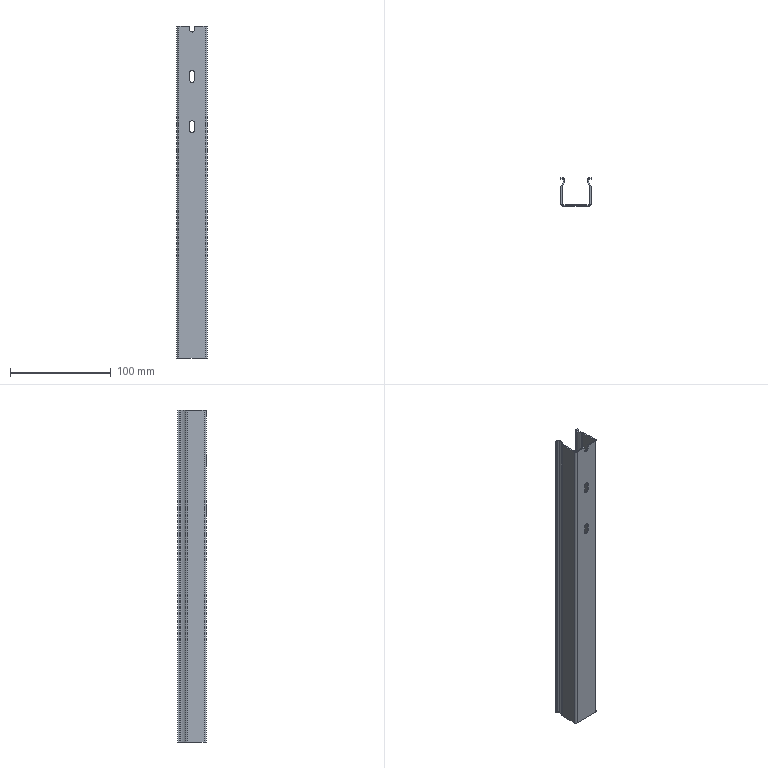Part | SolidWorks | features BaseBody 1 | 1 solid | 47 faces | box 30 x 28 x 330 mm | volume 35652 mm3 | cylinder 26 | plane 21 | commonest cylinder face diameters 5 x8 2 x3 4.5 x3 1.5 x2 3.5 x2 4 x2
STEP:
#1=CARTESIAN_POINT('',(-2.5,-12.75,-103.5));
#2=VERTEX_POINT('',#1);
#3=CARTESIAN_POINT('',(-2.5,-12.75,-96.5));
#4=VERTEX_POINT('',#3);
#5=CARTESIAN_POINT('',(-2.5,-12.75,-96.5));
#6=DIRECTION('',(0.,0.,1.));
#7=VECTOR('',#6,1000.);
#8=LINE('',#5,#7);
#9=EDGE_CURVE('',#2,#4,#8,.T.);
#10=ORIENTED_EDGE('',*,*,#9,.T.);
#11=CARTESIAN_POINT('',(-2.5,-14.,-96.5));
#12=VERTEX_POINT('',#11);
#13=CARTESIAN_POINT('',(-2.5,14.001,-96.5));
#14=DIRECTION('',(0.,-1.,0.));
#15=VECTOR('',#14,1000.);
#16=LINE('',#13,#15);
#17=EDGE_CURVE('',#4,#12,#16,.T.);
#18=ORIENTED_EDGE('',*,*,#17,.T.);
#19=CARTESIAN_POINT('',(-2.5,-14.,-103.5));
#20=VERTEX_POINT('',#19);
#21=CARTESIAN_POINT('',(-2.5,-14.,-96.5));
#22=DIRECTION('',(0.,0.,-1.));
#23=VECTOR('',#22,1000.);
#24=LINE('',#21,#23);
#25=EDGE_CURVE('',#12,#20,#24,.T.);
#26=ORIENTED_EDGE('',*,*,#25,.T.);
#27=CARTESIAN_POINT('',(-2.5,14.001,-103.5));
#28=DIRECTION('',(0.,-1.,0.));
#29=VECTOR('',#28,1000.);
#30=LINE('',#27,#29);
#31=EDGE_CURVE('',#2,#20,#30,.T.);
#32=ORIENTED_EDGE('',*,*,#31,.F.);
#33=EDGE_LOOP('',(#10,#18,#26,#32));
#34=FACE_OUTER_BOUND('',#33,.T.);
#35=CARTESIAN_POINT('',(-2.5,14.001,-96.5));
#36=DIRECTION('',(-1.,0.,0.));
#37=DIRECTION('',(0.,0.,1.));
#38=AXIS2_PLACEMENT_3D('',#35,#36,#37);
#39=PLANE('',#38);
#40=ADVANCED_FACE('',(#34),#39,.F.);
#41=CARTESIAN_POINT('',(0.,-12.75,-106.));
#42=VERTEX_POINT('',#41);
#43=CARTESIAN_POINT('',(0.,-14.,-106.));
#44=VERTEX_POINT('',#43);
#45=CARTESIAN_POINT('',(0.,14.001,-106.));
#46=DIRECTION('',(0.,-1.,0.));
#47=VECTOR('',#46,1000.);
#48=LINE('',#45,#47);
#49=EDGE_CURVE('',#42,#44,#48,.T.);
#50=ORIENTED_EDGE('',*,*,#49,.F.);
#51=CARTESIAN_POINT('',(0.,-12.75,-103.5));
#52=DIRECTION('',(0.,1.,0.));
#53=DIRECTION('',(0.,0.,-1.));
#54=AXIS2_PLACEMENT_3D('',#51,#52,#53);
#55=CIRCLE('',#54,2.5);
#56=EDGE_CURVE('',#42,#2,#55,.T.);
#57=ORIENTED_EDGE('',*,*,#56,.T.);
#58=ORIENTED_EDGE('',*,*,#31,.T.);
#59=CARTESIAN_POINT('',(0.,-14.,-103.5));
#60=DIRECTION('',(0.,-1.,0.));
#61=DIRECTION('',(0.,0.,-1.));
#62=AXIS2_PLACEMENT_3D('',#59,#60,#61);
#63=CIRCLE('',#62,2.5);
#64=EDGE_CURVE('',#20,#44,#63,.T.);
#65=ORIENTED_EDGE('',*,*,#64,.T.);
#66=EDGE_LOOP('',(#50,#57,#58,#65));
#67=FACE_OUTER_BOUND('',#66,.T.);
#68=CARTESIAN_POINT('',(0.,14.001,-103.5));
#69=DIRECTION('',(0.,-1.,0.));
#70=DIRECTION('',(0.,0.,-1.));
#71=AXIS2_PLACEMENT_3D('',#68,#69,#70);
#72=CYLINDRICAL_SURFACE('',#71,2.5);
#73=ADVANCED_FACE('',(#67),#72,.F.);
#74=CARTESIAN_POINT('',(2.5,-12.75,-96.5));
#75=VERTEX_POINT('',#74);
#76=CARTESIAN_POINT('',(2.5,-12.75,-103.5));
#77=VERTEX_POINT('',#76);
#78=CARTESIAN_POINT('',(2.5,-12.75,-96.5));
#79=DIRECTION('',(0.,0.,-1.));
#80=VECTOR('',#79,1000.);
#81=LINE('',#78,#80);
#82=EDGE_CURVE('',#75,#77,#81,.T.);
#83=ORIENTED_EDGE('',*,*,#82,.T.);
#84=CARTESIAN_POINT('',(2.5,-14.,-103.5));
#85=VERTEX_POINT('',#84);
#86=CARTESIAN_POINT('',(2.5,14.001,-103.5));
#87=DIRECTION('',(0.,-1.,0.));
#88=VECTOR('',#87,1000.);
#89=LINE('',#86,#88);
#90=EDGE_CURVE('',#77,#85,#89,.T.);
#91=ORIENTED_EDGE('',*,*,#90,.T.);
#92=CARTESIAN_POINT('',(2.5,-14.,-96.5));
#93=VERTEX_POINT('',#92);
#94=CARTESIAN_POINT('',(2.5,-14.,-96.5));
#95=DIRECTION('',(0.,0.,1.));
#96=VECTOR('',#95,1000.);
#97=LINE('',#94,#96);
#98=EDGE_CURVE('',#85,#93,#97,.T.);
#99=ORIENTED_EDGE('',*,*,#98,.T.);
#100=CARTESIAN_POINT('',(2.5,14.001,-96.5));
#101=DIRECTION('',(0.,-1.,0.));
#102=VECTOR('',#101,1000.);
#103=LINE('',#100,#102);
#104=EDGE_CURVE('',#75,#93,#103,.T.);
#105=ORIENTED_EDGE('',*,*,#104,.F.);
#106=EDGE_LOOP('',(#83,#91,#99,#105));
#107=FACE_OUTER_BOUND('',#106,.T.);
#108=CARTESIAN_POINT('',(2.5,14.001,-96.5));
#109=DIRECTION('',(1.,0.,0.));
#110=DIRECTION('',(0.,0.,1.));
#111=AXIS2_PLACEMENT_3D('',#108,#109,#110);
#112=PLANE('',#111);
#113=ADVANCED_FACE('',(#107),#112,.F.);
#114=CARTESIAN_POINT('',(0.,-12.75,-96.5));
#115=DIRECTION('',(0.,1.,0.));
#116=DIRECTION('',(0.,0.,-1.));
#117=AXIS2_PLACEMENT_3D('',#114,#115,#116);
#118=CIRCLE('',#117,2.5);
#119=EDGE_CURVE('',#4,#75,#118,.T.);
#120=ORIENTED_EDGE('',*,*,#119,.T.);
#121=ORIENTED_EDGE('',*,*,#104,.T.);
#122=CARTESIAN_POINT('',(0.,-14.,-96.5));
#123=DIRECTION('',(0.,-1.,0.));
#124=DIRECTION('',(0.,0.,-1.));
#125=AXIS2_PLACEMENT_3D('',#122,#123,#124);
#126=CIRCLE('',#125,2.5);
#127=EDGE_CURVE('',#93,#12,#126,.T.);
#128=ORIENTED_EDGE('',*,*,#127,.T.);
#129=ORIENTED_EDGE('',*,*,#17,.F.);
#130=EDGE_LOOP('',(#120,#121,#128,#129));
#131=FACE_OUTER_BOUND('',#130,.T.);
#132=CARTESIAN_POINT('',(0.,14.001,-96.5));
#133=DIRECTION('',(0.,-1.,0.));
#134=DIRECTION('',(0.,0.,-1.));
#135=AXIS2_PLACEMENT_3D('',#132,#133,#134);
#136=CYLINDRICAL_SURFACE('',#135,2.5);
#137=ADVANCED_FACE('',(#131),#136,.F.);
#138=CARTESIAN_POINT('',(-2.5,-12.75,-53.5));
#139=VERTEX_POINT('',#138);
#140=CARTESIAN_POINT('',(-2.5,-12.75,-46.5));
#141=VERTEX_POINT('',#140);
#142=CARTESIAN_POINT('',(-2.5,-12.75,-46.5));
#143=DIRECTION('',(0.,0.,1.));
#144=VECTOR('',#143,1000.);
#145=LINE('',#142,#144);
#146=EDGE_CURVE('',#139,#141,#145,.T.);
#147=ORIENTED_EDGE('',*,*,#146,.T.);
#148=CARTESIAN_POINT('',(-2.5,-14.,-46.5));
#149=VERTEX_POINT('',#148);
#150=CARTESIAN_POINT('',(-2.5,14.001,-46.5));
#151=DIRECTION('',(0.,-1.,0.));
#152=VECTOR('',#151,1000.);
#153=LINE('',#150,#152);
#154=EDGE_CURVE('',#141,#149,#153,.T.);
#155=ORIENTED_EDGE('',*,*,#154,.T.);
#156=CARTESIAN_POINT('',(-2.5,-14.,-53.5));
#157=VERTEX_POINT('',#156);
#158=CARTESIAN_POINT('',(-2.5,-14.,-46.5));
#159=DIRECTION('',(0.,0.,-1.));
#160=VECTOR('',#159,1000.);
#161=LINE('',#158,#160);
#162=EDGE_CURVE('',#149,#157,#161,.T.);
#163=ORIENTED_EDGE('',*,*,#162,.T.);
#164=CARTESIAN_POINT('',(-2.5,14.001,-53.5));
#165=DIRECTION('',(0.,-1.,0.));
#166=VECTOR('',#165,1000.);
#167=LINE('',#164,#166);
#168=EDGE_CURVE('',#139,#157,#167,.T.);
#169=ORIENTED_EDGE('',*,*,#168,.F.);
#170=EDGE_LOOP('',(#147,#155,#163,#169));
#171=FACE_OUTER_BOUND('',#170,.T.);
#172=CARTESIAN_POINT('',(-2.5,14.001,-46.5));
#173=DIRECTION('',(-1.,0.,0.));
#174=DIRECTION('',(0.,0.,1.));
#175=AXIS2_PLACEMENT_3D('',#172,#173,#174);
#176=PLANE('',#175);
#177=ADVANCED_FACE('',(#171),#176,.F.);
#178=CARTESIAN_POINT('',(0.,-12.75,-56.));
#179=VERTEX_POINT('',#178);
#180=CARTESIAN_POINT('',(0.,-14.,-56.));
#181=VERTEX_POINT('',#180);
#182=CARTESIAN_POINT('',(0.,14.001,-56.));
#183=DIRECTION('',(0.,-1.,0.));
#184=VECTOR('',#183,1000.);
#185=LINE('',#182,#184);
#186=EDGE_CURVE('',#179,#181,#185,.T.);
#187=ORIENTED_EDGE('',*,*,#186,.F.);
#188=CARTESIAN_POINT('',(0.,-12.75,-53.5));
#189=DIRECTION('',(0.,1.,0.));
#190=DIRECTION('',(0.,0.,-1.));
#191=AXIS2_PLACEMENT_3D('',#188,#189,#190);
#192=CIRCLE('',#191,2.5);
#193=EDGE_CURVE('',#179,#139,#192,.T.);
#194=ORIENTED_EDGE('',*,*,#193,.T.);
#195=ORIENTED_EDGE('',*,*,#168,.T.);
#196=CARTESIAN_POINT('',(0.,-14.,-53.5));
#197=DIRECTION('',(0.,-1.,0.));
#198=DIRECTION('',(0.,0.,-1.));
#199=AXIS2_PLACEMENT_3D('',#196,#197,#198);
#200=CIRCLE('',#199,2.5);
#201=EDGE_CURVE('',#157,#181,#200,.T.);
#202=ORIENTED_EDGE('',*,*,#201,.T.);
#203=EDGE_LOOP('',(#187,#194,#195,#202));
#204=FACE_OUTER_BOUND('',#203,.T.);
#205=CARTESIAN_POINT('',(0.,14.001,-53.5));
#206=DIRECTION('',(0.,-1.,0.));
#207=DIRECTION('',(0.,0.,-1.));
#208=AXIS2_PLACEMENT_3D('',#205,#206,#207);
#209=CYLINDRICAL_SURFACE('',#208,2.5);
#210=ADVANCED_FACE('',(#204),#209,.F.);
#211=CARTESIAN_POINT('',(2.5,-12.75,-46.5));
#212=VERTEX_POINT('',#211);
#213=CARTESIAN_POINT('',(2.5,-12.75,-53.5));
#214=VERTEX_POINT('',#213);
#215=CARTESIAN_POINT('',(2.5,-12.75,-46.5));
#216=DIRECTION('',(0.,0.,-1.));
#217=VECTOR('',#216,1000.);
#218=LINE('',#215,#217);
#219=EDGE_CURVE('',#212,#214,#218,.T.);
#220=ORIENTED_EDGE('',*,*,#219,.T.);
#221=CARTESIAN_POINT('',(2.5,-14.,-53.5));
#222=VERTEX_POINT('',#221);
#223=CARTESIAN_POINT('',(2.5,14.001,-53.5));
#224=DIRECTION('',(0.,-1.,0.));
#225=VECTOR('',#224,1000.);
#226=LINE('',#223,#225);
#227=EDGE_CURVE('',#214,#222,#226,.T.);
#228=ORIENTED_EDGE('',*,*,#227,.T.);
#229=CARTESIAN_POINT('',(2.5,-14.,-46.5));
#230=VERTEX_POINT('',#229);
#231=CARTESIAN_POINT('',(2.5,-14.,-46.5));
#232=DIRECTION('',(0.,0.,1.));
#233=VECTOR('',#232,1000.);
#234=LINE('',#231,#233);
#235=EDGE_CURVE('',#222,#230,#234,.T.);
#236=ORIENTED_EDGE('',*,*,#235,.T.);
#237=CARTESIAN_POINT('',(2.5,14.001,-46.5));
#238=DIRECTION('',(0.,-1.,0.));
#239=VECTOR('',#238,1000.);
#240=LINE('',#237,#239);
#241=EDGE_CURVE('',#212,#230,#240,.T.);
#242=ORIENTED_EDGE('',*,*,#241,.F.);
#243=EDGE_LOOP('',(#220,#228,#236,#242));
#244=FACE_OUTER_BOUND('',#243,.T.);
#245=CARTESIAN_POINT('',(2.5,14.001,-46.5));
#246=DIRECTION('',(1.,0.,0.));
#247=DIRECTION('',(0.,0.,1.));
#248=AXIS2_PLACEMENT_3D('',#245,#246,#247);
#249=PLANE('',#248);
#250=ADVANCED_FACE('',(#244),#249,.F.);
#251=CARTESIAN_POINT('',(0.,-12.75,-46.5));
#252=DIRECTION('',(0.,1.,0.));
#253=DIRECTION('',(0.,0.,-1.));
#254=AXIS2_PLACEMENT_3D('',#251,#252,#253);
#255=CIRCLE('',#254,2.5);
#256=EDGE_CURVE('',#141,#212,#255,.T.);
#257=ORIENTED_EDGE('',*,*,#256,.T.);
#258=ORIENTED_EDGE('',*,*,#241,.T.);
#259=CARTESIAN_POINT('',(0.,-14.,-46.5));
#260=DIRECTION('',(0.,-1.,0.));
#261=DIRECTION('',(0.,0.,-1.));
#262=AXIS2_PLACEMENT_3D('',#259,#260,#261);
#263=CIRCLE('',#262,2.5);
#264=EDGE_CURVE('',#230,#149,#263,.T.);
#265=ORIENTED_EDGE('',*,*,#264,.T.);
#266=ORIENTED_EDGE('',*,*,#154,.F.);
#267=EDGE_LOOP('',(#257,#258,#265,#266));
#268=FACE_OUTER_BOUND('',#267,.T.);
#269=CARTESIAN_POINT('',(0.,14.001,-46.5));
#270=DIRECTION('',(0.,-1.,0.));
#271=DIRECTION('',(0.,0.,-1.));
#272=AXIS2_PLACEMENT_3D('',#269,#270,#271);
#273=CYLINDRICAL_SURFACE('',#272,2.5);
#274=ADVANCED_FACE('',(#268),#273,.F.);
#275=CARTESIAN_POINT('',(-2.5,-14.,0.));
#276=VERTEX_POINT('',#275);
#277=CARTESIAN_POINT('',(-2.5,-14.,-3.5));
#278=VERTEX_POINT('',#277);
#279=CARTESIAN_POINT('',(-2.5,-14.,3.5));
#280=DIRECTION('',(0.,0.,-1.));
#281=VECTOR('',#280,1000.);
#282=LINE('',#279,#281);
#283=EDGE_CURVE('',#276,#278,#282,.T.);
#284=ORIENTED_EDGE('',*,*,#283,.T.);
#285=CARTESIAN_POINT('',(-2.5,-12.75,-3.5));
#286=VERTEX_POINT('',#285);
#287=CARTESIAN_POINT('',(-2.5,14.001,-3.5));
#288=DIRECTION('',(0.,-1.,0.));
#289=VECTOR('',#288,1000.);
#290=LINE('',#287,#289);
#291=EDGE_CURVE('',#286,#278,#290,.T.);
#292=ORIENTED_EDGE('',*,*,#291,.F.);
#293=CARTESIAN_POINT('',(-2.5,-12.75,0.));
#294=VERTEX_POINT('',#293);
#295=CARTESIAN_POINT('',(-2.5,-12.75,3.5));
#296=DIRECTION('',(0.,0.,1.));
#297=VECTOR('',#296,1000.);
#298=LINE('',#295,#297);
#299=EDGE_CURVE('',#286,#294,#298,.T.);
#300=ORIENTED_EDGE('',*,*,#299,.T.);
#301=CARTESIAN_POINT('',(-2.5,14.001,0.));
#302=DIRECTION('',(0.,1.,0.));
#303=VECTOR('',#302,1000.);
#304=LINE('',#301,#303);
#305=EDGE_CURVE('',#276,#294,#304,.T.);
#306=ORIENTED_EDGE('',*,*,#305,.F.);
#307=EDGE_LOOP('',(#284,#292,#300,#306));
#308=FACE_OUTER_BOUND('',#307,.T.);
#309=CARTESIAN_POINT('',(-2.5,14.001,3.5));
#310=DIRECTION('',(-1.,0.,0.));
#311=DIRECTION('',(0.,0.,1.));
#312=AXIS2_PLACEMENT_3D('',#309,#310,#311);
#313=PLANE('',#312);
#314=ADVANCED_FACE('',(#308),#313,.F.);
#315=CARTESIAN_POINT('',(2.5,-12.75,0.));
#316=VERTEX_POINT('',#315);
#317=CARTESIAN_POINT('',(2.5,-12.75,-3.5));
#318=VERTEX_POINT('',#317);
#319=CARTESIAN_POINT('',(2.5,-12.75,3.5));
#320=DIRECTION('',(0.,0.,-1.));
#321=VECTOR('',#320,1000.);
#322=LINE('',#319,#321);
#323=EDGE_CURVE('',#316,#318,#322,.T.);
#324=ORIENTED_EDGE('',*,*,#323,.T.);
#325=CARTESIAN_POINT('',(2.5,-14.,-3.5));
#326=VERTEX_POINT('',#325);
#327=CARTESIAN_POINT('',(2.5,14.001,-3.5));
#328=DIRECTION('',(0.,-1.,0.));
#329=VECTOR('',#328,1000.);
#330=LINE('',#327,#329);
#331=EDGE_CURVE('',#318,#326,#330,.T.);
#332=ORIENTED_EDGE('',*,*,#331,.T.);
#333=CARTESIAN_POINT('',(2.5,-14.,0.));
#334=VERTEX_POINT('',#333);
#335=CARTESIAN_POINT('',(2.5,-14.,3.5));
#336=DIRECTION('',(0.,0.,1.));
#337=VECTOR('',#336,1000.);
#338=LINE('',#335,#337);
#339=EDGE_CURVE('',#326,#334,#338,.T.);
#340=ORIENTED_EDGE('',*,*,#339,.T.);
#341=CARTESIAN_POINT('',(2.5,14.001,0.));
#342=DIRECTION('',(0.,-1.,0.));
#343=VECTOR('',#342,1000.);
#344=LINE('',#341,#343);
#345=EDGE_CURVE('',#316,#334,#344,.T.);
#346=ORIENTED_EDGE('',*,*,#345,.F.);
#347=EDGE_LOOP('',(#324,#332,#340,#346));
#348=FACE_OUTER_BOUND('',#347,.T.);
#349=CARTESIAN_POINT('',(2.5,14.001,3.5));
#350=DIRECTION('',(1.,0.,0.));
#351=DIRECTION('',(0.,0.,1.));
#352=AXIS2_PLACEMENT_3D('',#349,#350,#351);
#353=PLANE('',#352);
#354=ADVANCED_FACE('',(#348),#353,.F.);
#355=CARTESIAN_POINT('',(0.,-12.75,-6.));
#356=VERTEX_POINT('',#355);
#357=CARTESIAN_POINT('',(0.,-14.,-6.));
#358=VERTEX_POINT('',#357);
#359=CARTESIAN_POINT('',(0.,14.001,-6.));
#360=DIRECTION('',(0.,-1.,0.));
#361=VECTOR('',#360,1000.);
#362=LINE('',#359,#361);
#363=EDGE_CURVE('',#356,#358,#362,.T.);
#364=ORIENTED_EDGE('',*,*,#363,.F.);
#365=CARTESIAN_POINT('',(0.,-12.75,-3.5));
#366=DIRECTION('',(0.,1.,0.));
#367=DIRECTION('',(0.,0.,-1.));
#368=AXIS2_PLACEMENT_3D('',#365,#366,#367);
#369=CIRCLE('',#368,2.5);
#370=EDGE_CURVE('',#356,#286,#369,.T.);
#371=ORIENTED_EDGE('',*,*,#370,.T.);
#372=ORIENTED_EDGE('',*,*,#291,.T.);
#373=CARTESIAN_POINT('',(0.,-14.,-3.5));
#374=DIRECTION('',(0.,-1.,0.));
#375=DIRECTION('',(0.,0.,-1.));
#376=AXIS2_PLACEMENT_3D('',#373,#374,#375);
#377=CIRCLE('',#376,2.5);
#378=EDGE_CURVE('',#278,#358,#377,.T.);
#379=ORIENTED_EDGE('',*,*,#378,.T.);
#380=EDGE_LOOP('',(#364,#371,#372,#379));
#381=FACE_OUTER_BOUND('',#380,.T.);
#382=CARTESIAN_POINT('',(0.,14.001,-3.5));
#383=DIRECTION('',(0.,-1.,0.));
#384=DIRECTION('',(0.,0.,-1.));
#385=AXIS2_PLACEMENT_3D('',#382,#383,#384);
#386=CYLINDRICAL_SURFACE('',#385,2.5);
#387=ADVANCED_FACE('',(#381),#386,.F.);
#388=CARTESIAN_POINT('',(-13.,-12.75,-330.));
#389=VERTEX_POINT('',#388);
#390=CARTESIAN_POINT('',(-13.75,-12.,-330.));
#391=VERTEX_POINT('',#390);
#392=CARTESIAN_POINT('',(-13.,-12.,-330.));
#393=DIRECTION('',(0.,0.,-1.));
#394=DIRECTION('',(1.,0.,0.));
#395=AXIS2_PLACEMENT_3D('',#392,#393,#394);
#396=CIRCLE('',#395,0.75);
#397=EDGE_CURVE('',#389,#391,#396,.T.);
#398=ORIENTED_EDGE('',*,*,#397,.T.);
#399=CARTESIAN_POINT('',(-13.75,-12.,0.));
#400=VERTEX_POINT('',#399);
#401=CARTESIAN_POINT('',(-13.75,-12.,-330.));
#402=DIRECTION('',(0.,0.,1.));
#403=VECTOR('',#402,1000.);
#404=LINE('',#401,#403);
#405=EDGE_CURVE('',#391,#400,#404,.T.);
#406=ORIENTED_EDGE('',*,*,#405,.T.);
#407=CARTESIAN_POINT('',(-13.,-12.75,0.));
#408=VERTEX_POINT('',#407);
#409=CARTESIAN_POINT('',(-13.,-12.,0.));
#410=DIRECTION('',(0.,0.,1.));
#411=DIRECTION('',(1.,0.,0.));
#412=AXIS2_PLACEMENT_3D('',#409,#410,#411);
#413=CIRCLE('',#412,0.75);
#414=EDGE_CURVE('',#400,#408,#413,.T.);
#415=ORIENTED_EDGE('',*,*,#414,.T.);
#416=CARTESIAN_POINT('',(-13.,-12.75,-330.));
#417=DIRECTION('',(0.,0.,-1.));
#418=VECTOR('',#417,1000.);
#419=LINE('',#416,#418);
#420=EDGE_CURVE('',#408,#389,#419,.T.);
#421=ORIENTED_EDGE('',*,*,#420,.T.);
#422=EDGE_LOOP('',(#398,#406,#415,#421));
#423=FACE_OUTER_BOUND('',#422,.T.);
#424=CARTESIAN_POINT('',(-13.,-12.,-330.));
#425=DIRECTION('',(0.,0.,1.));
#426=DIRECTION('',(1.,0.,0.));
#427=AXIS2_PLACEMENT_3D('',#424,#425,#426);
#428=CYLINDRICAL_SURFACE('',#427,0.75);
#429=ADVANCED_FACE('',(#423),#428,.F.);
#430=CARTESIAN_POINT('',(13.75,-12.,-330.));
#431=VERTEX_POINT('',#430);
#432=CARTESIAN_POINT('',(13.,-12.75,-330.));
#433=VERTEX_POINT('',#432);
#434=CARTESIAN_POINT('',(13.,-12.,-330.));
#435=DIRECTION('',(0.,0.,-1.));
#436=DIRECTION('',(1.,0.,0.));
#437=AXIS2_PLACEMENT_3D('',#434,#435,#436);
#438=CIRCLE('',#437,0.75);
#439=EDGE_CURVE('',#431,#433,#438,.T.);
#440=ORIENTED_EDGE('',*,*,#439,.T.);
#441=CARTESIAN_POINT('',(13.,-12.75,0.));
#442=VERTEX_POINT('',#441);
#443=CARTESIAN_POINT('',(13.,-12.75,-330.));
#444=DIRECTION('',(0.,0.,1.));
#445=VECTOR('',#444,1000.);
#446=LINE('',#443,#445);
#447=EDGE_CURVE('',#433,#442,#446,.T.);
#448=ORIENTED_EDGE('',*,*,#447,.T.);
#449=CARTESIAN_POINT('',(13.75,-12.,0.));
#450=VERTEX_POINT('',#449);
#451=CARTESIAN_POINT('',(13.,-12.,0.));
#452=DIRECTION('',(0.,0.,1.));
#453=DIRECTION('',(1.,0.,0.));
#454=AXIS2_PLACEMENT_3D('',#451,#452,#453);
#455=CIRCLE('',#454,0.75);
#456=EDGE_CURVE('',#442,#450,#455,.T.);
#457=ORIENTED_EDGE('',*,*,#456,.T.);
#458=CARTESIAN_POINT('',(13.75,-12.,-330.));
#459=DIRECTION('',(0.,0.,-1.));
#460=VECTOR('',#459,1000.);
#461=LINE('',#458,#460);
#462=EDGE_CURVE('',#450,#431,#461,.T.);
#463=ORIENTED_EDGE('',*,*,#462,.T.);
#464=EDGE_LOOP('',(#440,#448,#457,#463));
#465=FACE_OUTER_BOUND('',#464,.T.);
#466=CARTESIAN_POINT('',(13.,-12.,-330.));
#467=DIRECTION('',(0.,0.,1.));
#468=DIRECTION('',(1.,0.,0.));
#469=AXIS2_PLACEMENT_3D('',#466,#467,#468);
#470=CYLINDRICAL_SURFACE('',#469,0.75);
#471=ADVANCED_FACE('',(#465),#470,.F.);
#472=CARTESIAN_POINT('',(13.439,5.746,-330.));
#473=VERTEX_POINT('',#472);
#474=CARTESIAN_POINT('',(13.75,4.75,-330.));
#475=VERTEX_POINT('',#474);
#476=CARTESIAN_POINT('',(12.,4.75,-330.));
#477=DIRECTION('',(0.,0.,-1.));
#478=DIRECTION('',(1.,0.,0.));
#479=AXIS2_PLACEMENT_3D('',#476,#477,#478);
#480=CIRCLE('',#479,1.75);
#481=EDGE_CURVE('',#473,#475,#480,.T.);
#482=ORIENTED_EDGE('',*,*,#481,.T.);
#483=CARTESIAN_POINT('',(13.75,4.75,0.));
#484=VERTEX_POINT('',#483);
#485=CARTESIAN_POINT('',(13.75,4.75,-330.));
#486=DIRECTION('',(0.,0.,1.));
#487=VECTOR('',#486,1000.);
#488=LINE('',#485,#487);
#489=EDGE_CURVE('',#475,#484,#488,.T.);
#490=ORIENTED_EDGE('',*,*,#489,.T.);
#491=CARTESIAN_POINT('',(13.439,5.746,0.));
#492=VERTEX_POINT('',#491);
#493=CARTESIAN_POINT('',(12.,4.75,0.));
#494=DIRECTION('',(0.,0.,1.));
#495=DIRECTION('',(1.,0.,0.));
#496=AXIS2_PLACEMENT_3D('',#493,#494,#495);
#497=CIRCLE('',#496,1.75);
#498=EDGE_CURVE('',#484,#492,#497,.T.);
#499=ORIENTED_EDGE('',*,*,#498,.T.);
#500=CARTESIAN_POINT('',(13.439,5.746,-330.));
#501=DIRECTION('',(0.,0.,-1.));
#502=VECTOR('',#501,1000.);
#503=LINE('',#500,#502);
#504=EDGE_CURVE('',#492,#473,#503,.T.);
#505=ORIENTED_EDGE('',*,*,#504,.T.);
#506=EDGE_LOOP('',(#482,#490,#499,#505));
#507=FACE_OUTER_BOUND('',#506,.T.);
#508=CARTESIAN_POINT('',(12.,4.75,-330.));
#509=DIRECTION('',(0.,0.,1.));
#510=DIRECTION('',(1.,0.,0.));
#511=AXIS2_PLACEMENT_3D('',#508,#509,#510);
#512=CYLINDRICAL_SURFACE('',#511,1.75);
#513=ADVANCED_FACE('',(#507),#512,.F.);
#514=CARTESIAN_POINT('',(-13.75,4.75,-330.));
#515=VERTEX_POINT('',#514);
#516=CARTESIAN_POINT('',(-13.439,5.746,-330.));
#517=VERTEX_POINT('',#516);
#518=CARTESIAN_POINT('',(-12.,4.75,-330.));
#519=DIRECTION('',(0.,0.,-1.));
#520=DIRECTION('',(1.,0.,0.));
#521=AXIS2_PLACEMENT_3D('',#518,#519,#520);
#522=CIRCLE('',#521,1.75);
#523=EDGE_CURVE('',#515,#517,#522,.T.);
#524=ORIENTED_EDGE('',*,*,#523,.T.);
#525=CARTESIAN_POINT('',(-13.439,5.746,0.));
#526=VERTEX_POINT('',#525);
#527=CARTESIAN_POINT('',(-13.439,5.746,-330.));
#528=DIRECTION('',(0.,0.,1.));
#529=VECTOR('',#528,1000.);
#530=LINE('',#527,#529);
#531=EDGE_CURVE('',#517,#526,#530,.T.);
#532=ORIENTED_EDGE('',*,*,#531,.T.);
#533=CARTESIAN_POINT('',(-13.75,4.75,0.));
#534=VERTEX_POINT('',#533);
#535=CARTESIAN_POINT('',(-12.,4.75,0.));
#536=DIRECTION('',(0.,0.,1.));
#537=DIRECTION('',(1.,0.,0.));
#538=AXIS2_PLACEMENT_3D('',#535,#536,#537);
#539=CIRCLE('',#538,1.75);
#540=EDGE_CURVE('',#526,#534,#539,.T.);
#541=ORIENTED_EDGE('',*,*,#540,.T.);
#542=CARTESIAN_POINT('',(-13.75,4.75,-330.));
#543=DIRECTION('',(0.,0.,-1.));
#544=VECTOR('',#543,1000.);
#545=LINE('',#542,#544);
#546=EDGE_CURVE('',#534,#515,#545,.T.);
#547=ORIENTED_EDGE('',*,*,#546,.T.);
#548=EDGE_LOOP('',(#524,#532,#541,#547));
#549=FACE_OUTER_BOUND('',#548,.T.);
#550=CARTESIAN_POINT('',(-12.,4.75,-330.));
#551=DIRECTION('',(0.,0.,1.));
#552=DIRECTION('',(1.,0.,0.));
#553=AXIS2_PLACEMENT_3D('',#550,#551,#552);
#554=CYLINDRICAL_SURFACE('',#553,1.75);
#555=ADVANCED_FACE('',(#549),#554,.F.);
#556=CARTESIAN_POINT('',(13.55,14.,-330.));
#557=VERTEX_POINT('',#556);
#558=CARTESIAN_POINT('',(11.311,11.526,-330.));
#559=VERTEX_POINT('',#558);
#560=CARTESIAN_POINT('',(13.55,11.75,-330.));
#561=DIRECTION('',(0.,0.,1.));
#562=DIRECTION('',(1.,0.,0.));
#563=AXIS2_PLACEMENT_3D('',#560,#561,#562);
#564=CIRCLE('',#563,2.25);
#565=EDGE_CURVE('',#557,#559,#564,.T.);
#566=ORIENTED_EDGE('',*,*,#565,.T.);
#567=CARTESIAN_POINT('',(11.311,11.526,0.));
#568=VERTEX_POINT('',#567);
#569=CARTESIAN_POINT('',(11.311,11.526,-330.));
#570=DIRECTION('',(0.,0.,1.));
#571=VECTOR('',#570,1000.);
#572=LINE('',#569,#571);
#573=EDGE_CURVE('',#559,#568,#572,.T.);
#574=ORIENTED_EDGE('',*,*,#573,.T.);
#575=CARTESIAN_POINT('',(13.55,14.,0.));
#576=VERTEX_POINT('',#575);
#577=CARTESIAN_POINT('',(13.55,11.75,0.));
#578=DIRECTION('',(0.,0.,-1.));
#579=DIRECTION('',(1.,0.,0.));
#580=AXIS2_PLACEMENT_3D('',#577,#578,#579);
#581=CIRCLE('',#580,2.25);
#582=EDGE_CURVE('',#568,#576,#581,.T.);
#583=ORIENTED_EDGE('',*,*,#582,.T.);
#584=CARTESIAN_POINT('',(13.55,14.,-330.));
#585=DIRECTION('',(0.,0.,-1.));
#586=VECTOR('',#585,1000.);
#587=LINE('',#584,#586);
#588=EDGE_CURVE('',#576,#557,#587,.T.);
#589=ORIENTED_EDGE('',*,*,#588,.T.);
#590=EDGE_LOOP('',(#566,#574,#583,#589));
#591=FACE_OUTER_BOUND('',#590,.T.);
#592=CARTESIAN_POINT('',(13.55,11.75,-330.));
#593=DIRECTION('',(0.,0.,1.));
#594=DIRECTION('',(1.,0.,0.));
#595=AXIS2_PLACEMENT_3D('',#592,#593,#594);
#596=CYLINDRICAL_SURFACE('',#595,2.25);
#597=ADVANCED_FACE('',(#591),#596,.T.);
#598=CARTESIAN_POINT('',(-11.3,11.75,-330.));
#599=VERTEX_POINT('',#598);
#600=CARTESIAN_POINT('',(-11.3,11.75,0.));
#601=VERTEX_POINT('',#600);
#602=CARTESIAN_POINT('',(-11.3,11.75,-330.));
#603=DIRECTION('',(0.,0.,1.));
#604=VECTOR('',#603,1000.);
#605=LINE('',#602,#604);
#606=EDGE_CURVE('',#599,#601,#605,.T.);
#607=ORIENTED_EDGE('',*,*,#606,.F.);
#608=CARTESIAN_POINT('',(-13.55,14.,-330.));
#609=VERTEX_POINT('',#608);
#610=CARTESIAN_POINT('',(-13.55,11.75,-330.));
#611=DIRECTION('',(0.,0.,1.));
#612=DIRECTION('',(1.,0.,0.));
#613=AXIS2_PLACEMENT_3D('',#610,#611,#612);
#614=CIRCLE('',#613,2.25);
#615=EDGE_CURVE('',#599,#609,#614,.T.);
#616=ORIENTED_EDGE('',*,*,#615,.T.);
#617=CARTESIAN_POINT('',(-13.55,14.,0.));
#618=VERTEX_POINT('',#617);
#619=CARTESIAN_POINT('',(-13.55,14.,-330.));
#620=DIRECTION('',(0.,0.,1.));
#621=VECTOR('',#620,1000.);
#622=LINE('',#619,#621);
#623=EDGE_CURVE('',#609,#618,#622,.T.);
#624=ORIENTED_EDGE('',*,*,#623,.T.);
#625=CARTESIAN_POINT('',(-13.55,11.75,0.));
#626=DIRECTION('',(0.,0.,-1.));
#627=DIRECTION('',(1.,0.,0.));
#628=AXIS2_PLACEMENT_3D('',#625,#626,#627);
#629=CIRCLE('',#628,2.25);
#630=EDGE_CURVE('',#618,#601,#629,.T.);
#631=ORIENTED_EDGE('',*,*,#630,.T.);
#632=EDGE_LOOP('',(#607,#616,#624,#631));
#633=FACE_OUTER_BOUND('',#632,.T.);
#634=CARTESIAN_POINT('',(-13.55,11.75,-330.));
#635=DIRECTION('',(0.,0.,1.));
#636=DIRECTION('',(1.,0.,0.));
#637=AXIS2_PLACEMENT_3D('',#634,#635,#636);
#638=CYLINDRICAL_SURFACE('',#637,2.25);
#639=ADVANCED_FACE('',(#633),#638,.T.);
#640=CARTESIAN_POINT('',(-11.311,11.526,-330.));
#641=VERTEX_POINT('',#640);
#642=CARTESIAN_POINT('',(-23.55,12.75,-330.));
#643=DIRECTION('',(0.,0.,1.));
#644=DIRECTION('',(1.,0.,0.));
#645=AXIS2_PLACEMENT_3D('',#642,#643,#644);
#646=CIRCLE('',#645,12.3);
#647=EDGE_CURVE('',#517,#641,#646,.T.);
#648=ORIENTED_EDGE('',*,*,#647,.T.);
#649=CARTESIAN_POINT('',(-11.311,11.526,0.));
#650=VERTEX_POINT('',#649);
#651=CARTESIAN_POINT('',(-11.311,11.526,-330.));
#652=DIRECTION('',(0.,0.,-1.));
#653=VECTOR('',#652,1000.);
#654=LINE('',#651,#653);
#655=EDGE_CURVE('',#650,#641,#654,.T.);
#656=ORIENTED_EDGE('',*,*,#655,.F.);
#657=CARTESIAN_POINT('',(-23.55,12.75,0.));
#658=DIRECTION('',(0.,0.,1.));
#659=DIRECTION('',(1.,0.,0.));
#660=AXIS2_PLACEMENT_3D('',#657,#658,#659);
#661=CIRCLE('',#660,12.3);
#662=EDGE_CURVE('',#526,#650,#661,.T.);
#663=ORIENTED_EDGE('',*,*,#662,.F.);
#664=ORIENTED_EDGE('',*,*,#531,.F.);
#665=EDGE_LOOP('',(#648,#656,#663,#664));
#666=FACE_OUTER_BOUND('',#665,.T.);
#667=CARTESIAN_POINT('',(-23.55,12.75,-330.));
#668=DIRECTION('',(0.,0.,1.));
#669=DIRECTION('',(1.,0.,0.));
#670=AXIS2_PLACEMENT_3D('',#667,#668,#669);
#671=CYLINDRICAL_SURFACE('',#670,12.3);
#672=ADVANCED_FACE('',(#666),#671,.T.);
#673=CARTESIAN_POINT('',(23.55,12.75,0.));
#674=DIRECTION('',(0.,0.,1.));
#675=DIRECTION('',(1.,0.,0.));
#676=AXIS2_PLACEMENT_3D('',#673,#674,#675);
#677=CIRCLE('',#676,12.3);
#678=EDGE_CURVE('',#568,#492,#677,.T.);
#679=ORIENTED_EDGE('',*,*,#678,.F.);
#680=ORIENTED_EDGE('',*,*,#573,.F.);
#681=CARTESIAN_POINT('',(23.55,12.75,-330.));
#682=DIRECTION('',(0.,0.,1.));
#683=DIRECTION('',(1.,0.,0.));
#684=AXIS2_PLACEMENT_3D('',#681,#682,#683);
#685=CIRCLE('',#684,12.3);
#686=EDGE_CURVE('',#559,#473,#685,.T.);
#687=ORIENTED_EDGE('',*,*,#686,.T.);
#688=ORIENTED_EDGE('',*,*,#504,.F.);
#689=EDGE_LOOP('',(#679,#680,#687,#688));
#690=FACE_OUTER_BOUND('',#689,.T.);
#691=CARTESIAN_POINT('',(23.55,12.75,-330.));
#692=DIRECTION('',(0.,0.,1.));
#693=DIRECTION('',(1.,0.,0.));
#694=AXIS2_PLACEMENT_3D('',#691,#692,#693);
#695=CYLINDRICAL_SURFACE('',#694,12.3);
#696=ADVANCED_FACE('',(#690),#695,.T.);
#697=ORIENTED_EDGE('',*,*,#219,.F.);
#698=ORIENTED_EDGE('',*,*,#256,.F.);
#699=ORIENTED_EDGE('',*,*,#146,.F.);
#700=ORIENTED_EDGE('',*,*,#193,.F.);
#701=CARTESIAN_POINT('',(0.,-12.75,-53.5));
#702=DIRECTION('',(0.,1.,0.));
#703=DIRECTION('',(0.,0.,-1.));
#704=AXIS2_PLACEMENT_3D('',#701,#702,#703);
#705=CIRCLE('',#704,2.5);
#706=EDGE_CURVE('',#214,#179,#705,.T.);
#707=ORIENTED_EDGE('',*,*,#706,.F.);
#708=EDGE_LOOP('',(#697,#698,#699,#700,#707));
#709=FACE_BOUND('',#708,.T.);
#710=ORIENTED_EDGE('',*,*,#82,.F.);
#711=ORIENTED_EDGE('',*,*,#119,.F.);
#712=ORIENTED_EDGE('',*,*,#9,.F.);
#713=ORIENTED_EDGE('',*,*,#56,.F.);
#714=CARTESIAN_POINT('',(0.,-12.75,-103.5));
#715=DIRECTION('',(0.,1.,0.));
#716=DIRECTION('',(0.,0.,-1.));
#717=AXIS2_PLACEMENT_3D('',#714,#715,#716);
#718=CIRCLE('',#717,2.5);
#719=EDGE_CURVE('',#77,#42,#718,.T.);
#720=ORIENTED_EDGE('',*,*,#719,.F.);
#721=EDGE_LOOP('',(#710,#711,#712,#713,#720));
#722=FACE_BOUND('',#721,.T.);
#723=CARTESIAN_POINT('',(0.,-12.75,-3.5));
#724=DIRECTION('',(0.,1.,0.));
#725=DIRECTION('',(0.,0.,-1.));
#726=AXIS2_PLACEMENT_3D('',#723,#724,#725);
#727=CIRCLE('',#726,2.5);
#728=EDGE_CURVE('',#318,#356,#727,.T.);
#729=ORIENTED_EDGE('',*,*,#728,.F.);
#730=ORIENTED_EDGE('',*,*,#323,.F.);
#731=CARTESIAN_POINT('',(0.,-12.75,0.));
#732=DIRECTION('',(1.,0.,0.));
#733=VECTOR('',#732,1000.);
#734=LINE('',#731,#733);
#735=EDGE_CURVE('',#316,#442,#734,.T.);
#736=ORIENTED_EDGE('',*,*,#735,.T.);
#737=ORIENTED_EDGE('',*,*,#447,.F.);
#738=CARTESIAN_POINT('',(0.,-12.75,-330.));
#739=DIRECTION('',(1.,0.,0.));
#740=VECTOR('',#739,1000.);
#741=LINE('',#738,#740);
#742=EDGE_CURVE('',#389,#433,#741,.T.);
#743=ORIENTED_EDGE('',*,*,#742,.F.);
#744=ORIENTED_EDGE('',*,*,#420,.F.);
#745=CARTESIAN_POINT('',(0.,-12.75,0.));
#746=DIRECTION('',(1.,0.,0.));
#747=VECTOR('',#746,1000.);
#748=LINE('',#745,#747);
#749=EDGE_CURVE('',#408,#294,#748,.T.);
#750=ORIENTED_EDGE('',*,*,#749,.T.);
#751=ORIENTED_EDGE('',*,*,#299,.F.);
#752=ORIENTED_EDGE('',*,*,#370,.F.);
#753=EDGE_LOOP('',(#729,#730,#736,#737,#743,#744,#750,#751,#752));
#754=FACE_OUTER_BOUND('',#753,.T.);
#755=CARTESIAN_POINT('',(-15.,-12.75,-330.));
#756=DIRECTION('',(0.,-1.,0.));
#757=DIRECTION('',(0.,0.,-1.));
#758=AXIS2_PLACEMENT_3D('',#755,#756,#757);
#759=PLANE('',#758);
#760=ADVANCED_FACE('',(#709,#722,#754),#759,.F.);
#761=CARTESIAN_POINT('',(13.75,0.,0.));
#762=DIRECTION('',(0.,1.,0.));
#763=VECTOR('',#762,1000.);
#764=LINE('',#761,#763);
#765=EDGE_CURVE('',#450,#484,#764,.T.);
#766=ORIENTED_EDGE('',*,*,#765,.T.);
#767=ORIENTED_EDGE('',*,*,#489,.F.);
#768=CARTESIAN_POINT('',(13.75,0.,-330.));
#769=DIRECTION('',(0.,1.,0.));
#770=VECTOR('',#769,1000.);
#771=LINE('',#768,#770);
#772=EDGE_CURVE('',#431,#475,#771,.T.);
#773=ORIENTED_EDGE('',*,*,#772,.F.);
#774=ORIENTED_EDGE('',*,*,#462,.F.);
#775=EDGE_LOOP('',(#766,#767,#773,#774));
#776=FACE_OUTER_BOUND('',#775,.T.);
#777=CARTESIAN_POINT('',(13.75,14.,-330.));
#778=DIRECTION('',(1.,0.,0.));
#779=DIRECTION('',(0.,1.,0.));
#780=AXIS2_PLACEMENT_3D('',#777,#778,#779);
#781=PLANE('',#780);
#782=ADVANCED_FACE('',(#776),#781,.F.);
#783=CARTESIAN_POINT('',(-13.75,0.,-330.));
#784=DIRECTION('',(0.,-1.,0.));
#785=VECTOR('',#784,1000.);
#786=LINE('',#783,#785);
#787=EDGE_CURVE('',#515,#391,#786,.T.);
#788=ORIENTED_EDGE('',*,*,#787,.F.);
#789=ORIENTED_EDGE('',*,*,#546,.F.);
#790=CARTESIAN_POINT('',(-13.75,0.,0.));
#791=DIRECTION('',(0.,-1.,0.));
#792=VECTOR('',#791,1000.);
#793=LINE('',#790,#792);
#794=EDGE_CURVE('',#534,#400,#793,.T.);
#795=ORIENTED_EDGE('',*,*,#794,.T.);
#796=ORIENTED_EDGE('',*,*,#405,.F.);
#797=EDGE_LOOP('',(#788,#789,#795,#796));
#798=FACE_OUTER_BOUND('',#797,.T.);
#799=CARTESIAN_POINT('',(-13.75,14.,-330.));
#800=DIRECTION('',(-1.,0.,0.));
#801=DIRECTION('',(0.,1.,0.));
#802=AXIS2_PLACEMENT_3D('',#799,#800,#801);
#803=PLANE('',#802);
#804=ADVANCED_FACE('',(#798),#803,.F.);
#805=CARTESIAN_POINT('',(-13.,-14.,-330.));
#806=VERTEX_POINT('',#805);
#807=CARTESIAN_POINT('',(-15.,-12.,-330.));
#808=VERTEX_POINT('',#807);
#809=CARTESIAN_POINT('',(-13.,-12.,-330.));
#810=DIRECTION('',(0.,0.,-1.));
#811=DIRECTION('',(1.,0.,0.));
#812=AXIS2_PLACEMENT_3D('',#809,#810,#811);
#813=CIRCLE('',#812,2.);
#814=EDGE_CURVE('',#806,#808,#813,.T.);
#815=ORIENTED_EDGE('',*,*,#814,.F.);
#816=CARTESIAN_POINT('',(-13.,-14.,0.));
#817=VERTEX_POINT('',#816);
#818=CARTESIAN_POINT('',(-13.,-14.,-330.));
#819=DIRECTION('',(0.,0.,-1.));
#820=VECTOR('',#819,1000.);
#821=LINE('',#818,#820);
#822=EDGE_CURVE('',#817,#806,#821,.T.);
#823=ORIENTED_EDGE('',*,*,#822,.F.);
#824=CARTESIAN_POINT('',(-15.,-12.,0.));
#825=VERTEX_POINT('',#824);
#826=CARTESIAN_POINT('',(-13.,-12.,0.));
#827=DIRECTION('',(0.,0.,1.));
#828=DIRECTION('',(1.,0.,0.));
#829=AXIS2_PLACEMENT_3D('',#826,#827,#828);
#830=CIRCLE('',#829,2.);
#831=EDGE_CURVE('',#825,#817,#830,.T.);
#832=ORIENTED_EDGE('',*,*,#831,.F.);
#833=CARTESIAN_POINT('',(-15.,-12.,-330.));
#834=DIRECTION('',(0.,0.,1.));
#835=VECTOR('',#834,1000.);
#836=LINE('',#833,#835);
#837=EDGE_CURVE('',#808,#825,#836,.T.);
#838=ORIENTED_EDGE('',*,*,#837,.F.);
#839=EDGE_LOOP('',(#815,#823,#832,#838));
#840=FACE_OUTER_BOUND('',#839,.T.);
#841=CARTESIAN_POINT('',(-13.,-12.,-330.));
#842=DIRECTION('',(0.,0.,1.));
#843=DIRECTION('',(1.,0.,0.));
#844=AXIS2_PLACEMENT_3D('',#841,#842,#843);
#845=CYLINDRICAL_SURFACE('',#844,2.);
#846=ADVANCED_FACE('',(#840),#845,.T.);
#847=CARTESIAN_POINT('',(15.,-12.,-330.));
#848=VERTEX_POINT('',#847);
#849=CARTESIAN_POINT('',(13.,-14.,-330.));
#850=VERTEX_POINT('',#849);
#851=CARTESIAN_POINT('',(13.,-12.,-330.));
#852=DIRECTION('',(0.,0.,-1.));
#853=DIRECTION('',(1.,0.,0.));
#854=AXIS2_PLACEMENT_3D('',#851,#852,#853);
#855=CIRCLE('',#854,2.);
#856=EDGE_CURVE('',#848,#850,#855,.T.);
#857=ORIENTED_EDGE('',*,*,#856,.F.);
#858=CARTESIAN_POINT('',(15.,-12.,0.));
#859=VERTEX_POINT('',#858);
#860=CARTESIAN_POINT('',(15.,-12.,-330.));
#861=DIRECTION('',(0.,0.,-1.));
#862=VECTOR('',#861,1000.);
#863=LINE('',#860,#862);
#864=EDGE_CURVE('',#859,#848,#863,.T.);
#865=ORIENTED_EDGE('',*,*,#864,.F.);
#866=CARTESIAN_POINT('',(13.,-14.,0.));
#867=VERTEX_POINT('',#866);
#868=CARTESIAN_POINT('',(13.,-12.,0.));
#869=DIRECTION('',(0.,0.,1.));
#870=DIRECTION('',(1.,0.,0.));
#871=AXIS2_PLACEMENT_3D('',#868,#869,#870);
#872=CIRCLE('',#871,2.);
#873=EDGE_CURVE('',#867,#859,#872,.T.);
#874=ORIENTED_EDGE('',*,*,#873,.F.);
#875=CARTESIAN_POINT('',(13.,-14.,-330.));
#876=DIRECTION('',(0.,0.,1.));
#877=VECTOR('',#876,1000.);
#878=LINE('',#875,#877);
#879=EDGE_CURVE('',#850,#867,#878,.T.);
#880=ORIENTED_EDGE('',*,*,#879,.F.);
#881=EDGE_LOOP('',(#857,#865,#874,#880));
#882=FACE_OUTER_BOUND('',#881,.T.);
#883=CARTESIAN_POINT('',(13.,-12.,-330.));
#884=DIRECTION('',(0.,0.,1.));
#885=DIRECTION('',(1.,0.,0.));
#886=AXIS2_PLACEMENT_3D('',#883,#884,#885);
#887=CYLINDRICAL_SURFACE('',#886,2.);
#888=ADVANCED_FACE('',(#882),#887,.T.);
#889=CARTESIAN_POINT('',(14.466,6.458,-330.));
#890=VERTEX_POINT('',#889);
#891=CARTESIAN_POINT('',(15.,4.75,-330.));
#892=VERTEX_POINT('',#891);
#893=CARTESIAN_POINT('',(12.,4.75,-330.));
#894=DIRECTION('',(0.,0.,-1.));
#895=DIRECTION('',(1.,0.,0.));
#896=AXIS2_PLACEMENT_3D('',#893,#894,#895);
#897=CIRCLE('',#896,3.);
#898=EDGE_CURVE('',#890,#892,#897,.T.);
#899=ORIENTED_EDGE('',*,*,#898,.F.);
#900=CARTESIAN_POINT('',(14.466,6.458,0.));
#901=VERTEX_POINT('',#900);
#902=CARTESIAN_POINT('',(14.466,6.458,-330.));
#903=DIRECTION('',(0.,0.,-1.));
#904=VECTOR('',#903,1000.);
#905=LINE('',#902,#904);
#906=EDGE_CURVE('',#901,#890,#905,.T.);
#907=ORIENTED_EDGE('',*,*,#906,.F.);
#908=CARTESIAN_POINT('',(15.,4.75,0.));
#909=VERTEX_POINT('',#908);
#910=CARTESIAN_POINT('',(12.,4.75,0.));
#911=DIRECTION('',(0.,0.,1.));
#912=DIRECTION('',(1.,0.,0.));
#913=AXIS2_PLACEMENT_3D('',#910,#911,#912);
#914=CIRCLE('',#913,3.);
#915=EDGE_CURVE('',#909,#901,#914,.T.);
#916=ORIENTED_EDGE('',*,*,#915,.F.);
#917=CARTESIAN_POINT('',(15.,4.75,0.));
#918=DIRECTION('',(0.,0.,1.));
#919=VECTOR('',#918,1000.);
#920=LINE('',#917,#919);
#921=EDGE_CURVE('',#892,#909,#920,.T.);
#922=ORIENTED_EDGE('',*,*,#921,.F.);
#923=EDGE_LOOP('',(#899,#907,#916,#922));
#924=FACE_OUTER_BOUND('',#923,.T.);
#925=CARTESIAN_POINT('',(12.,4.75,-330.));
#926=DIRECTION('',(0.,0.,1.));
#927=DIRECTION('',(1.,0.,0.));
#928=AXIS2_PLACEMENT_3D('',#925,#926,#927);
#929=CYLINDRICAL_SURFACE('',#928,3.);
#930=ADVANCED_FACE('',(#924),#929,.T.);
#931=CARTESIAN_POINT('',(-15.,4.75,-330.));
#932=VERTEX_POINT('',#931);
#933=CARTESIAN_POINT('',(-14.466,6.458,-330.));
#934=VERTEX_POINT('',#933);
#935=CARTESIAN_POINT('',(-12.,4.75,-330.));
#936=DIRECTION('',(0.,0.,-1.));
#937=DIRECTION('',(1.,0.,0.));
#938=AXIS2_PLACEMENT_3D('',#935,#936,#937);
#939=CIRCLE('',#938,3.);
#940=EDGE_CURVE('',#932,#934,#939,.T.);
#941=ORIENTED_EDGE('',*,*,#940,.F.);
#942=CARTESIAN_POINT('',(-15.,4.75,0.));
#943=VERTEX_POINT('',#942);
#944=CARTESIAN_POINT('',(-15.,4.75,-330.));
#945=DIRECTION('',(0.,0.,-1.));
#946=VECTOR('',#945,1000.);
#947=LINE('',#944,#946);
#948=EDGE_CURVE('',#943,#932,#947,.T.);
#949=ORIENTED_EDGE('',*,*,#948,.F.);
#950=CARTESIAN_POINT('',(-14.466,6.458,0.));
#951=VERTEX_POINT('',#950);
#952=CARTESIAN_POINT('',(-12.,4.75,0.));
#953=DIRECTION('',(0.,0.,1.));
#954=DIRECTION('',(1.,0.,0.));
#955=AXIS2_PLACEMENT_3D('',#952,#953,#954);
#956=CIRCLE('',#955,3.);
#957=EDGE_CURVE('',#951,#943,#956,.T.);
#958=ORIENTED_EDGE('',*,*,#957,.F.);
#959=CARTESIAN_POINT('',(-14.466,6.458,-330.));
#960=DIRECTION('',(0.,0.,1.));
#961=VECTOR('',#960,1000.);
#962=LINE('',#959,#961);
#963=EDGE_CURVE('',#934,#951,#962,.T.);
#964=ORIENTED_EDGE('',*,*,#963,.F.);
#965=EDGE_LOOP('',(#941,#949,#958,#964));
#966=FACE_OUTER_BOUND('',#965,.T.);
#967=CARTESIAN_POINT('',(-12.,4.75,-330.));
#968=DIRECTION('',(0.,0.,1.));
#969=DIRECTION('',(1.,0.,0.));
#970=AXIS2_PLACEMENT_3D('',#967,#968,#969);
#971=CYLINDRICAL_SURFACE('',#970,3.);
#972=ADVANCED_FACE('',(#966),#971,.T.);
#973=CARTESIAN_POINT('',(13.55,12.75,-330.));
#974=VERTEX_POINT('',#973);
#975=CARTESIAN_POINT('',(12.555,11.65,-330.));
#976=VERTEX_POINT('',#975);
#977=CARTESIAN_POINT('',(13.55,11.75,-330.));
#978=DIRECTION('',(0.,0.,1.));
#979=DIRECTION('',(1.,0.,0.));
#980=AXIS2_PLACEMENT_3D('',#977,#978,#979);
#981=CIRCLE('',#980,1.);
#982=EDGE_CURVE('',#974,#976,#981,.T.);
#983=ORIENTED_EDGE('',*,*,#982,.F.);
#984=CARTESIAN_POINT('',(13.55,12.75,0.));
#985=VERTEX_POINT('',#984);
#986=CARTESIAN_POINT('',(13.55,12.75,-330.));
#987=DIRECTION('',(0.,0.,-1.));
#988=VECTOR('',#987,1000.);
#989=LINE('',#986,#988);
#990=EDGE_CURVE('',#985,#974,#989,.T.);
#991=ORIENTED_EDGE('',*,*,#990,.F.);
#992=CARTESIAN_POINT('',(12.555,11.65,0.));
#993=VERTEX_POINT('',#992);
#994=CARTESIAN_POINT('',(13.55,11.75,0.));
#995=DIRECTION('',(0.,0.,-1.));
#996=DIRECTION('',(1.,0.,0.));
#997=AXIS2_PLACEMENT_3D('',#994,#995,#996);
#998=CIRCLE('',#997,1.);
#999=EDGE_CURVE('',#993,#985,#998,.T.);
#1000=ORIENTED_EDGE('',*,*,#999,.F.);
#1001=CARTESIAN_POINT('',(12.555,11.65,-330.));
#1002=DIRECTION('',(0.,0.,1.));
#1003=VECTOR('',#1002,1000.);
#1004=LINE('',#1001,#1003);
#1005=EDGE_CURVE('',#976,#993,#1004,.T.);
#1006=ORIENTED_EDGE('',*,*,#1005,.F.);
#1007=EDGE_LOOP('',(#983,#991,#1000,#1006));
#1008=FACE_OUTER_BOUND('',#1007,.T.);
#1009=CARTESIAN_POINT('',(13.55,11.75,-330.));
#1010=DIRECTION('',(0.,0.,1.));
#1011=DIRECTION('',(1.,0.,0.));
#1012=AXIS2_PLACEMENT_3D('',#1009,#1010,#1011);
#1013=CYLINDRICAL_SURFACE('',#1012,1.);
#1014=ADVANCED_FACE('',(#1008),#1013,.F.);
#1015=CARTESIAN_POINT('',(-12.55,11.75,-330.));
#1016=VERTEX_POINT('',#1015);
#1017=CARTESIAN_POINT('',(-12.55,11.75,0.));
#1018=VERTEX_POINT('',#1017);
#1019=CARTESIAN_POINT('',(-12.55,11.75,-330.));
#1020=DIRECTION('',(0.,0.,1.));
#1021=VECTOR('',#1020,1000.);
#1022=LINE('',#1019,#1021);
#1023=EDGE_CURVE('',#1016,#1018,#1022,.T.);
#1024=ORIENTED_EDGE('',*,*,#1023,.F.);
#1025=CARTESIAN_POINT('',(-12.555,11.65,-330.));
#1026=VERTEX_POINT('',#1025);
#1027=CARTESIAN_POINT('',(-13.55,11.75,-330.));
#1028=DIRECTION('',(0.,0.,1.));
#1029=DIRECTION('',(1.,0.,0.));
#1030=AXIS2_PLACEMENT_3D('',#1027,#1028,#1029);
#1031=CIRCLE('',#1030,1.);
#1032=EDGE_CURVE('',#1026,#1016,#1031,.T.);
#1033=ORIENTED_EDGE('',*,*,#1032,.F.);
#1034=CARTESIAN_POINT('',(-12.555,11.65,0.));
#1035=VERTEX_POINT('',#1034);
#1036=CARTESIAN_POINT('',(-12.555,11.65,-330.));
#1037=DIRECTION('',(0.,0.,-1.));
#1038=VECTOR('',#1037,1000.);
#1039=LINE('',#1036,#1038);
#1040=EDGE_CURVE('',#1035,#1026,#1039,.T.);
#1041=ORIENTED_EDGE('',*,*,#1040,.F.);
#1042=CARTESIAN_POINT('',(-13.55,11.75,0.));
#1043=DIRECTION('',(0.,0.,-1.));
#1044=DIRECTION('',(1.,0.,0.));
#1045=AXIS2_PLACEMENT_3D('',#1042,#1043,#1044);
#1046=CIRCLE('',#1045,1.);
#1047=EDGE_CURVE('',#1018,#1035,#1046,.T.);
#1048=ORIENTED_EDGE('',*,*,#1047,.F.);
#1049=EDGE_LOOP('',(#1024,#1033,#1041,#1048));
#1050=FACE_OUTER_BOUND('',#1049,.T.);
#1051=CARTESIAN_POINT('',(-13.55,11.75,-330.));
#1052=DIRECTION('',(0.,0.,1.));
#1053=DIRECTION('',(1.,0.,0.));
#1054=AXIS2_PLACEMENT_3D('',#1051,#1052,#1053);
#1055=CYLINDRICAL_SURFACE('',#1054,1.);
#1056=ADVANCED_FACE('',(#1050),#1055,.F.);
#1057=CARTESIAN_POINT('',(-13.55,12.75,-330.));
#1058=VERTEX_POINT('',#1057);
#1059=CARTESIAN_POINT('',(-15.,12.75,-330.));
#1060=VERTEX_POINT('',#1059);
#1061=CARTESIAN_POINT('',(-15.,12.75,-330.));
#1062=DIRECTION('',(-1.,0.,0.));
#1063=VECTOR('',#1062,1000.);
#1064=LINE('',#1061,#1063);
#1065=EDGE_CURVE('',#1058,#1060,#1064,.T.);
#1066=ORIENTED_EDGE('',*,*,#1065,.F.);
#1067=CARTESIAN_POINT('',(-13.55,12.75,0.));
#1068=VERTEX_POINT('',#1067);
#1069=CARTESIAN_POINT('',(-13.55,12.75,0.));
#1070=DIRECTION('',(0.,0.,1.));
#1071=VECTOR('',#1070,1000.);
#1072=LINE('',#1069,#1071);
#1073=EDGE_CURVE('',#1058,#1068,#1072,.T.);
#1074=ORIENTED_EDGE('',*,*,#1073,.T.);
#1075=CARTESIAN_POINT('',(-15.,12.75,0.));
#1076=VERTEX_POINT('',#1075);
#1077=CARTESIAN_POINT('',(-15.,12.75,0.));
#1078=DIRECTION('',(-1.,0.,0.));
#1079=VECTOR('',#1078,1000.);
#1080=LINE('',#1077,#1079);
#1081=EDGE_CURVE('',#1068,#1076,#1080,.T.);
#1082=ORIENTED_EDGE('',*,*,#1081,.T.);
#1083=CARTESIAN_POINT('',(-15.,12.75,-330.));
#1084=DIRECTION('',(0.,0.,1.));
#1085=VECTOR('',#1084,1000.);
#1086=LINE('',#1083,#1085);
#1087=EDGE_CURVE('',#1060,#1076,#1086,.T.);
#1088=ORIENTED_EDGE('',*,*,#1087,.F.);
#1089=EDGE_LOOP('',(#1066,#1074,#1082,#1088));
#1090=FACE_OUTER_BOUND('',#1089,.T.);
#1091=CARTESIAN_POINT('',(-15.,12.75,-330.));
#1092=DIRECTION('',(0.,1.,0.));
#1093=DIRECTION('',(1.,0.,0.));
#1094=AXIS2_PLACEMENT_3D('',#1091,#1092,#1093);
#1095=PLANE('',#1094);
#1096=ADVANCED_FACE('',(#1090),#1095,.F.);
#1097=CARTESIAN_POINT('',(-23.55,12.75,-330.));
#1098=DIRECTION('',(0.,0.,1.));
#1099=DIRECTION('',(-1.,0.,0.));
#1100=AXIS2_PLACEMENT_3D('',#1097,#1098,#1099);
#1101=CIRCLE('',#1100,11.05);
#1102=EDGE_CURVE('',#934,#1026,#1101,.T.);
#1103=ORIENTED_EDGE('',*,*,#1102,.F.);
#1104=ORIENTED_EDGE('',*,*,#963,.T.);
#1105=CARTESIAN_POINT('',(-23.55,12.75,0.));
#1106=DIRECTION('',(0.,0.,1.));
#1107=DIRECTION('',(-1.,0.,0.));
#1108=AXIS2_PLACEMENT_3D('',#1105,#1106,#1107);
#1109=CIRCLE('',#1108,11.05);
#1110=EDGE_CURVE('',#951,#1035,#1109,.T.);
#1111=ORIENTED_EDGE('',*,*,#1110,.T.);
#1112=ORIENTED_EDGE('',*,*,#1040,.T.);
#1113=EDGE_LOOP('',(#1103,#1104,#1111,#1112));
#1114=FACE_OUTER_BOUND('',#1113,.T.);
#1115=CARTESIAN_POINT('',(-23.55,12.75,-330.));
#1116=DIRECTION('',(0.,0.,1.));
#1117=DIRECTION('',(1.,0.,0.));
#1118=AXIS2_PLACEMENT_3D('',#1115,#1116,#1117);
#1119=CYLINDRICAL_SURFACE('',#1118,11.05);
#1120=ADVANCED_FACE('',(#1114),#1119,.F.);
#1121=CARTESIAN_POINT('',(15.,12.75,0.));
#1122=VERTEX_POINT('',#1121);
#1123=CARTESIAN_POINT('',(15.,12.75,0.));
#1124=DIRECTION('',(-1.,0.,0.));
#1125=VECTOR('',#1124,1000.);
#1126=LINE('',#1123,#1125);
#1127=EDGE_CURVE('',#1122,#985,#1126,.T.);
#1128=ORIENTED_EDGE('',*,*,#1127,.T.);
#1129=ORIENTED_EDGE('',*,*,#990,.T.);
#1130=CARTESIAN_POINT('',(15.,12.75,-330.));
#1131=VERTEX_POINT('',#1130);
#1132=CARTESIAN_POINT('',(15.,12.75,-330.));
#1133=DIRECTION('',(-1.,0.,0.));
#1134=VECTOR('',#1133,1000.);
#1135=LINE('',#1132,#1134);
#1136=EDGE_CURVE('',#1131,#974,#1135,.T.);
#1137=ORIENTED_EDGE('',*,*,#1136,.F.);
#1138=CARTESIAN_POINT('',(15.,12.75,-330.));
#1139=DIRECTION('',(0.,0.,1.));
#1140=VECTOR('',#1139,1000.);
#1141=LINE('',#1138,#1140);
#1142=EDGE_CURVE('',#1131,#1122,#1141,.T.);
#1143=ORIENTED_EDGE('',*,*,#1142,.T.);
#1144=EDGE_LOOP('',(#1128,#1129,#1137,#1143));
#1145=FACE_OUTER_BOUND('',#1144,.T.);
#1146=CARTESIAN_POINT('',(15.,12.75,-330.));
#1147=DIRECTION('',(0.,1.,0.));
#1148=DIRECTION('',(1.,0.,0.));
#1149=AXIS2_PLACEMENT_3D('',#1146,#1147,#1148);
#1150=PLANE('',#1149);
#1151=ADVANCED_FACE('',(#1145),#1150,.F.);
#1152=CARTESIAN_POINT('',(23.55,12.75,0.));
#1153=DIRECTION('',(0.,0.,1.));
#1154=DIRECTION('',(1.,0.,0.));
#1155=AXIS2_PLACEMENT_3D('',#1152,#1153,#1154);
#1156=CIRCLE('',#1155,11.05);
#1157=EDGE_CURVE('',#993,#901,#1156,.T.);
#1158=ORIENTED_EDGE('',*,*,#1157,.T.);
#1159=ORIENTED_EDGE('',*,*,#906,.T.);
#1160=CARTESIAN_POINT('',(23.55,12.75,-330.));
#1161=DIRECTION('',(0.,0.,1.));
#1162=DIRECTION('',(1.,0.,0.));
#1163=AXIS2_PLACEMENT_3D('',#1160,#1161,#1162);
#1164=CIRCLE('',#1163,11.05);
#1165=EDGE_CURVE('',#976,#890,#1164,.T.);
#1166=ORIENTED_EDGE('',*,*,#1165,.F.);
#1167=ORIENTED_EDGE('',*,*,#1005,.T.);
#1168=EDGE_LOOP('',(#1158,#1159,#1166,#1167));
#1169=FACE_OUTER_BOUND('',#1168,.T.);
#1170=CARTESIAN_POINT('',(23.55,12.75,-330.));
#1171=DIRECTION('',(0.,0.,1.));
#1172=DIRECTION('',(1.,0.,0.));
#1173=AXIS2_PLACEMENT_3D('',#1170,#1171,#1172);
#1174=CYLINDRICAL_SURFACE('',#1173,11.05);
#1175=ADVANCED_FACE('',(#1169),#1174,.F.);
#1176=ORIENTED_EDGE('',*,*,#305,.T.);
#1177=ORIENTED_EDGE('',*,*,#749,.F.);
#1178=ORIENTED_EDGE('',*,*,#414,.F.);
#1179=ORIENTED_EDGE('',*,*,#794,.F.);
#1180=ORIENTED_EDGE('',*,*,#540,.F.);
#1181=ORIENTED_EDGE('',*,*,#662,.T.);
#1182=CARTESIAN_POINT('',(-13.55,11.75,0.));
#1183=DIRECTION('',(0.,0.,-1.));
#1184=DIRECTION('',(1.,0.,0.));
#1185=AXIS2_PLACEMENT_3D('',#1182,#1183,#1184);
#1186=CIRCLE('',#1185,2.25);
#1187=EDGE_CURVE('',#601,#650,#1186,.T.);
#1188=ORIENTED_EDGE('',*,*,#1187,.F.);
#1189=ORIENTED_EDGE('',*,*,#630,.F.);
#1190=CARTESIAN_POINT('',(-15.,14.,0.));
#1191=VERTEX_POINT('',#1190);
#1192=CARTESIAN_POINT('',(-15.,14.,0.));
#1193=DIRECTION('',(-1.,0.,0.));
#1194=VECTOR('',#1193,1000.);
#1195=LINE('',#1192,#1194);
#1196=EDGE_CURVE('',#618,#1191,#1195,.T.);
#1197=ORIENTED_EDGE('',*,*,#1196,.T.);
#1198=CARTESIAN_POINT('',(-15.,14.,0.));
#1199=DIRECTION('',(0.,-1.,0.));
#1200=VECTOR('',#1199,1000.);
#1201=LINE('',#1198,#1200);
#1202=EDGE_CURVE('',#1191,#1076,#1201,.T.);
#1203=ORIENTED_EDGE('',*,*,#1202,.T.);
#1204=ORIENTED_EDGE('',*,*,#1081,.F.);
#1205=CARTESIAN_POINT('',(-13.55,11.75,0.));
#1206=DIRECTION('',(0.,0.,-1.));
#1207=DIRECTION('',(1.,0.,0.));
#1208=AXIS2_PLACEMENT_3D('',#1205,#1206,#1207);
#1209=CIRCLE('',#1208,1.);
#1210=EDGE_CURVE('',#1068,#1018,#1209,.T.);
#1211=ORIENTED_EDGE('',*,*,#1210,.T.);
#1212=ORIENTED_EDGE('',*,*,#1047,.T.);
#1213=ORIENTED_EDGE('',*,*,#1110,.F.);
#1214=ORIENTED_EDGE('',*,*,#957,.T.);
#1215=CARTESIAN_POINT('',(-15.,14.,0.));
#1216=DIRECTION('',(0.,-1.,0.));
#1217=VECTOR('',#1216,1000.);
#1218=LINE('',#1215,#1217);
#1219=EDGE_CURVE('',#943,#825,#1218,.T.);
#1220=ORIENTED_EDGE('',*,*,#1219,.T.);
#1221=ORIENTED_EDGE('',*,*,#831,.T.);
#1222=CARTESIAN_POINT('',(-15.,-14.,0.));
#1223=DIRECTION('',(1.,0.,0.));
#1224=VECTOR('',#1223,1000.);
#1225=LINE('',#1222,#1224);
#1226=EDGE_CURVE('',#817,#276,#1225,.T.);
#1227=ORIENTED_EDGE('',*,*,#1226,.T.);
#1228=EDGE_LOOP('',(#1176,#1177,#1178,#1179,#1180,#1181,#1188,#1189,#1197,#1203,#1204,#1211,#1212,#1213,#1214,#1220,#1221,#1227));
#1229=FACE_OUTER_BOUND('',#1228,.T.);
#1230=CARTESIAN_POINT('',(0.,0.,0.));
#1231=DIRECTION('',(0.,0.,1.));
#1232=DIRECTION('',(1.,0.,0.));
#1233=AXIS2_PLACEMENT_3D('',#1230,#1231,#1232);
#1234=PLANE('',#1233);
#1235=ADVANCED_FACE('',(#1229),#1234,.T.);
#1236=ORIENTED_EDGE('',*,*,#588,.F.);
#1237=CARTESIAN_POINT('',(15.,14.,0.));
#1238=VERTEX_POINT('',#1237);
#1239=CARTESIAN_POINT('',(-15.,14.,0.));
#1240=DIRECTION('',(-1.,0.,0.));
#1241=VECTOR('',#1240,1000.);
#1242=LINE('',#1239,#1241);
#1243=EDGE_CURVE('',#1238,#576,#1242,.T.);
#1244=ORIENTED_EDGE('',*,*,#1243,.F.);
#1245=CARTESIAN_POINT('',(15.,14.,-330.));
#1246=VERTEX_POINT('',#1245);
#1247=CARTESIAN_POINT('',(15.,14.,-330.));
#1248=DIRECTION('',(0.,0.,1.));
#1249=VECTOR('',#1248,1000.);
#1250=LINE('',#1247,#1249);
#1251=EDGE_CURVE('',#1246,#1238,#1250,.T.);
#1252=ORIENTED_EDGE('',*,*,#1251,.F.);
#1253=CARTESIAN_POINT('',(-15.,14.,-330.));
#1254=DIRECTION('',(-1.,0.,0.));
#1255=VECTOR('',#1254,1000.);
#1256=LINE('',#1253,#1255);
#1257=EDGE_CURVE('',#1246,#557,#1256,.T.);
#1258=ORIENTED_EDGE('',*,*,#1257,.T.);
#1259=EDGE_LOOP('',(#1236,#1244,#1252,#1258));
#1260=FACE_OUTER_BOUND('',#1259,.T.);
#1261=CARTESIAN_POINT('',(-15.,14.,-330.));
#1262=DIRECTION('',(0.,1.,0.));
#1263=DIRECTION('',(1.,0.,0.));
#1264=AXIS2_PLACEMENT_3D('',#1261,#1262,#1263);
#1265=PLANE('',#1264);
#1266=ADVANCED_FACE('',(#1260),#1265,.T.);
#1267=ORIENTED_EDGE('',*,*,#1087,.T.);
#1268=ORIENTED_EDGE('',*,*,#1202,.F.);
#1269=CARTESIAN_POINT('',(-15.,14.,-330.));
#1270=VERTEX_POINT('',#1269);
#1271=CARTESIAN_POINT('',(-15.,14.,-330.));
#1272=DIRECTION('',(0.,0.,1.));
#1273=VECTOR('',#1272,1000.);
#1274=LINE('',#1271,#1273);
#1275=EDGE_CURVE('',#1270,#1191,#1274,.T.);
#1276=ORIENTED_EDGE('',*,*,#1275,.F.);
#1277=CARTESIAN_POINT('',(-15.,14.,-330.));
#1278=DIRECTION('',(0.,-1.,0.));
#1279=VECTOR('',#1278,1000.);
#1280=LINE('',#1277,#1279);
#1281=EDGE_CURVE('',#1270,#1060,#1280,.T.);
#1282=ORIENTED_EDGE('',*,*,#1281,.T.);
#1283=EDGE_LOOP('',(#1267,#1268,#1276,#1282));
#1284=FACE_OUTER_BOUND('',#1283,.T.);
#1285=CARTESIAN_POINT('',(-15.,14.,-330.));
#1286=DIRECTION('',(-1.,0.,0.));
#1287=DIRECTION('',(0.,1.,0.));
#1288=AXIS2_PLACEMENT_3D('',#1285,#1286,#1287);
#1289=PLANE('',#1288);
#1290=ADVANCED_FACE('',(#1284),#1289,.T.);
#1291=ORIENTED_EDGE('',*,*,#264,.F.);
#1292=ORIENTED_EDGE('',*,*,#235,.F.);
#1293=CARTESIAN_POINT('',(0.,-14.,-53.5));
#1294=DIRECTION('',(0.,-1.,0.));
#1295=DIRECTION('',(0.,0.,-1.));
#1296=AXIS2_PLACEMENT_3D('',#1293,#1294,#1295);
#1297=CIRCLE('',#1296,2.5);
#1298=EDGE_CURVE('',#181,#222,#1297,.T.);
#1299=ORIENTED_EDGE('',*,*,#1298,.F.);
#1300=ORIENTED_EDGE('',*,*,#201,.F.);
#1301=ORIENTED_EDGE('',*,*,#162,.F.);
#1302=EDGE_LOOP('',(#1291,#1292,#1299,#1300,#1301));
#1303=FACE_BOUND('',#1302,.T.);
#1304=ORIENTED_EDGE('',*,*,#127,.F.);
#1305=ORIENTED_EDGE('',*,*,#98,.F.);
#1306=CARTESIAN_POINT('',(0.,-14.,-103.5));
#1307=DIRECTION('',(0.,-1.,0.));
#1308=DIRECTION('',(0.,0.,-1.));
#1309=AXIS2_PLACEMENT_3D('',#1306,#1307,#1308);
#1310=CIRCLE('',#1309,2.5);
#1311=EDGE_CURVE('',#44,#85,#1310,.T.);
#1312=ORIENTED_EDGE('',*,*,#1311,.F.);
#1313=ORIENTED_EDGE('',*,*,#64,.F.);
#1314=ORIENTED_EDGE('',*,*,#25,.F.);
#1315=EDGE_LOOP('',(#1304,#1305,#1312,#1313,#1314));
#1316=FACE_BOUND('',#1315,.T.);
#1317=ORIENTED_EDGE('',*,*,#339,.F.);
#1318=CARTESIAN_POINT('',(0.,-14.,-3.5));
#1319=DIRECTION('',(0.,-1.,0.));
#1320=DIRECTION('',(0.,0.,-1.));
#1321=AXIS2_PLACEMENT_3D('',#1318,#1319,#1320);
#1322=CIRCLE('',#1321,2.5);
#1323=EDGE_CURVE('',#358,#326,#1322,.T.);
#1324=ORIENTED_EDGE('',*,*,#1323,.F.);
#1325=ORIENTED_EDGE('',*,*,#378,.F.);
#1326=ORIENTED_EDGE('',*,*,#283,.F.);
#1327=ORIENTED_EDGE('',*,*,#1226,.F.);
#1328=ORIENTED_EDGE('',*,*,#822,.T.);
#1329=CARTESIAN_POINT('',(-15.,-14.,-330.));
#1330=DIRECTION('',(1.,0.,0.));
#1331=VECTOR('',#1330,1000.);
#1332=LINE('',#1329,#1331);
#1333=EDGE_CURVE('',#806,#850,#1332,.T.);
#1334=ORIENTED_EDGE('',*,*,#1333,.T.);
#1335=ORIENTED_EDGE('',*,*,#879,.T.);
#1336=CARTESIAN_POINT('',(-15.,-14.,0.));
#1337=DIRECTION('',(1.,0.,0.));
#1338=VECTOR('',#1337,1000.);
#1339=LINE('',#1336,#1338);
#1340=EDGE_CURVE('',#334,#867,#1339,.T.);
#1341=ORIENTED_EDGE('',*,*,#1340,.F.);
#1342=EDGE_LOOP('',(#1317,#1324,#1325,#1326,#1327,#1328,#1334,#1335,#1341));
#1343=FACE_OUTER_BOUND('',#1342,.T.);
#1344=CARTESIAN_POINT('',(-15.,-14.,-330.));
#1345=DIRECTION('',(0.,-1.,0.));
#1346=DIRECTION('',(0.,0.,-1.));
#1347=AXIS2_PLACEMENT_3D('',#1344,#1345,#1346);
#1348=PLANE('',#1347);
#1349=ADVANCED_FACE('',(#1303,#1316,#1343),#1348,.T.);
#1350=ORIENTED_EDGE('',*,*,#1142,.F.);
#1351=CARTESIAN_POINT('',(15.,14.,-330.));
#1352=DIRECTION('',(0.,1.,0.));
#1353=VECTOR('',#1352,1000.);
#1354=LINE('',#1351,#1353);
#1355=EDGE_CURVE('',#1131,#1246,#1354,.T.);
#1356=ORIENTED_EDGE('',*,*,#1355,.T.);
#1357=ORIENTED_EDGE('',*,*,#1251,.T.);
#1358=CARTESIAN_POINT('',(15.,14.,0.));
#1359=DIRECTION('',(0.,1.,0.));
#1360=VECTOR('',#1359,1000.);
#1361=LINE('',#1358,#1360);
#1362=EDGE_CURVE('',#1122,#1238,#1361,.T.);
#1363=ORIENTED_EDGE('',*,*,#1362,.F.);
#1364=EDGE_LOOP('',(#1350,#1356,#1357,#1363));
#1365=FACE_OUTER_BOUND('',#1364,.T.);
#1366=CARTESIAN_POINT('',(15.,14.,-330.));
#1367=DIRECTION('',(1.,0.,0.));
#1368=DIRECTION('',(0.,1.,0.));
#1369=AXIS2_PLACEMENT_3D('',#1366,#1367,#1368);
#1370=PLANE('',#1369);
#1371=ADVANCED_FACE('',(#1365),#1370,.T.);
#1372=CARTESIAN_POINT('',(15.,14.,0.));
#1373=DIRECTION('',(0.,1.,0.));
#1374=VECTOR('',#1373,1000.);
#1375=LINE('',#1372,#1374);
#1376=EDGE_CURVE('',#859,#909,#1375,.T.);
#1377=ORIENTED_EDGE('',*,*,#1376,.F.);
#1378=ORIENTED_EDGE('',*,*,#864,.T.);
#1379=CARTESIAN_POINT('',(15.,14.,-330.));
#1380=DIRECTION('',(0.,1.,0.));
#1381=VECTOR('',#1380,1000.);
#1382=LINE('',#1379,#1381);
#1383=EDGE_CURVE('',#848,#892,#1382,.T.);
#1384=ORIENTED_EDGE('',*,*,#1383,.T.);
#1385=ORIENTED_EDGE('',*,*,#921,.T.);
#1386=EDGE_LOOP('',(#1377,#1378,#1384,#1385));
#1387=FACE_OUTER_BOUND('',#1386,.T.);
#1388=CARTESIAN_POINT('',(15.,14.,-330.));
#1389=DIRECTION('',(1.,0.,0.));
#1390=DIRECTION('',(0.,1.,0.));
#1391=AXIS2_PLACEMENT_3D('',#1388,#1389,#1390);
#1392=PLANE('',#1391);
#1393=ADVANCED_FACE('',(#1387),#1392,.T.);
#1394=CARTESIAN_POINT('',(-15.,14.,-330.));
#1395=DIRECTION('',(0.,-1.,0.));
#1396=VECTOR('',#1395,1000.);
#1397=LINE('',#1394,#1396);
#1398=EDGE_CURVE('',#932,#808,#1397,.T.);
#1399=ORIENTED_EDGE('',*,*,#1398,.T.);
#1400=ORIENTED_EDGE('',*,*,#837,.T.);
#1401=ORIENTED_EDGE('',*,*,#1219,.F.);
#1402=ORIENTED_EDGE('',*,*,#948,.T.);
#1403=EDGE_LOOP('',(#1399,#1400,#1401,#1402));
#1404=FACE_OUTER_BOUND('',#1403,.T.);
#1405=CARTESIAN_POINT('',(-15.,14.,-330.));
#1406=DIRECTION('',(-1.,0.,0.));
#1407=DIRECTION('',(0.,1.,0.));
#1408=AXIS2_PLACEMENT_3D('',#1405,#1406,#1407);
#1409=PLANE('',#1408);
#1410=ADVANCED_FACE('',(#1404),#1409,.T.);
#1411=CARTESIAN_POINT('',(-13.55,11.75,-330.));
#1412=DIRECTION('',(0.,0.,1.));
#1413=DIRECTION('',(1.,0.,0.));
#1414=AXIS2_PLACEMENT_3D('',#1411,#1412,#1413);
#1415=CIRCLE('',#1414,2.25);
#1416=EDGE_CURVE('',#641,#599,#1415,.T.);
#1417=ORIENTED_EDGE('',*,*,#1416,.F.);
#1418=ORIENTED_EDGE('',*,*,#647,.F.);
#1419=ORIENTED_EDGE('',*,*,#523,.F.);
#1420=ORIENTED_EDGE('',*,*,#787,.T.);
#1421=ORIENTED_EDGE('',*,*,#397,.F.);
#1422=ORIENTED_EDGE('',*,*,#742,.T.);
#1423=ORIENTED_EDGE('',*,*,#439,.F.);
#1424=ORIENTED_EDGE('',*,*,#772,.T.);
#1425=ORIENTED_EDGE('',*,*,#481,.F.);
#1426=ORIENTED_EDGE('',*,*,#686,.F.);
#1427=ORIENTED_EDGE('',*,*,#565,.F.);
#1428=ORIENTED_EDGE('',*,*,#1257,.F.);
#1429=ORIENTED_EDGE('',*,*,#1355,.F.);
#1430=ORIENTED_EDGE('',*,*,#1136,.T.);
#1431=ORIENTED_EDGE('',*,*,#982,.T.);
#1432=ORIENTED_EDGE('',*,*,#1165,.T.);
#1433=ORIENTED_EDGE('',*,*,#898,.T.);
#1434=ORIENTED_EDGE('',*,*,#1383,.F.);
#1435=ORIENTED_EDGE('',*,*,#856,.T.);
#1436=ORIENTED_EDGE('',*,*,#1333,.F.);
#1437=ORIENTED_EDGE('',*,*,#814,.T.);
#1438=ORIENTED_EDGE('',*,*,#1398,.F.);
#1439=ORIENTED_EDGE('',*,*,#940,.T.);
#1440=ORIENTED_EDGE('',*,*,#1102,.T.);
#1441=ORIENTED_EDGE('',*,*,#1032,.T.);
#1442=CARTESIAN_POINT('',(-13.55,11.75,-330.));
#1443=DIRECTION('',(0.,0.,1.));
#1444=DIRECTION('',(1.,0.,0.));
#1445=AXIS2_PLACEMENT_3D('',#1442,#1443,#1444);
#1446=CIRCLE('',#1445,1.);
#1447=EDGE_CURVE('',#1016,#1058,#1446,.T.);
#1448=ORIENTED_EDGE('',*,*,#1447,.T.);
#1449=ORIENTED_EDGE('',*,*,#1065,.T.);
#1450=ORIENTED_EDGE('',*,*,#1281,.F.);
#1451=CARTESIAN_POINT('',(-15.,14.,-330.));
#1452=DIRECTION('',(-1.,0.,0.));
#1453=VECTOR('',#1452,1000.);
#1454=LINE('',#1451,#1453);
#1455=EDGE_CURVE('',#609,#1270,#1454,.T.);
#1456=ORIENTED_EDGE('',*,*,#1455,.F.);
#1457=ORIENTED_EDGE('',*,*,#615,.F.);
#1458=EDGE_LOOP('',(#1417,#1418,#1419,#1420,#1421,#1422,#1423,#1424,#1425,#1426,#1427,#1428,#1429,#1430,#1431,#1432,#1433,#1434,#1435,#1436,#1437,#1438,#1439,#1440,#1441,#1448,#1449,#1450,#1456,#1457));
#1459=FACE_OUTER_BOUND('',#1458,.T.);
#1460=CARTESIAN_POINT('',(0.,0.,-330.));
#1461=DIRECTION('',(0.,0.,1.));
#1462=DIRECTION('',(1.,0.,0.));
#1463=AXIS2_PLACEMENT_3D('',#1460,#1461,#1462);
#1464=PLANE('',#1463);
#1465=ADVANCED_FACE('',(#1459),#1464,.F.);
#1466=ORIENTED_EDGE('',*,*,#623,.F.);
#1467=ORIENTED_EDGE('',*,*,#1455,.T.);
#1468=ORIENTED_EDGE('',*,*,#1275,.T.);
#1469=ORIENTED_EDGE('',*,*,#1196,.F.);
#1470=EDGE_LOOP('',(#1466,#1467,#1468,#1469));
#1471=FACE_OUTER_BOUND('',#1470,.T.);
#1472=CARTESIAN_POINT('',(-15.,14.,-330.));
#1473=DIRECTION('',(0.,1.,0.));
#1474=DIRECTION('',(1.,0.,0.));
#1475=AXIS2_PLACEMENT_3D('',#1472,#1473,#1474);
#1476=PLANE('',#1475);
#1477=ADVANCED_FACE('',(#1471),#1476,.T.);
#1478=ORIENTED_EDGE('',*,*,#345,.T.);
#1479=ORIENTED_EDGE('',*,*,#1340,.T.);
#1480=ORIENTED_EDGE('',*,*,#873,.T.);
#1481=ORIENTED_EDGE('',*,*,#1376,.T.);
#1482=ORIENTED_EDGE('',*,*,#915,.T.);
#1483=ORIENTED_EDGE('',*,*,#1157,.F.);
#1484=ORIENTED_EDGE('',*,*,#999,.T.);
#1485=ORIENTED_EDGE('',*,*,#1127,.F.);
#1486=ORIENTED_EDGE('',*,*,#1362,.T.);
#1487=ORIENTED_EDGE('',*,*,#1243,.T.);
#1488=ORIENTED_EDGE('',*,*,#582,.F.);
#1489=ORIENTED_EDGE('',*,*,#678,.T.);
#1490=ORIENTED_EDGE('',*,*,#498,.F.);
#1491=ORIENTED_EDGE('',*,*,#765,.F.);
#1492=ORIENTED_EDGE('',*,*,#456,.F.);
#1493=ORIENTED_EDGE('',*,*,#735,.F.);
#1494=EDGE_LOOP('',(#1478,#1479,#1480,#1481,#1482,#1483,#1484,#1485,#1486,#1487,#1488,#1489,#1490,#1491,#1492,#1493));
#1495=FACE_OUTER_BOUND('',#1494,.T.);
#1496=CARTESIAN_POINT('',(0.,0.,0.));
#1497=DIRECTION('',(0.,0.,1.));
#1498=DIRECTION('',(1.,0.,0.));
#1499=AXIS2_PLACEMENT_3D('',#1496,#1497,#1498);
#1500=PLANE('',#1499);
#1501=ADVANCED_FACE('',(#1495),#1500,.T.);
#1502=ORIENTED_EDGE('',*,*,#1447,.F.);
#1503=ORIENTED_EDGE('',*,*,#1023,.T.);
#1504=ORIENTED_EDGE('',*,*,#1210,.F.);
#1505=ORIENTED_EDGE('',*,*,#1073,.F.);
#1506=EDGE_LOOP('',(#1502,#1503,#1504,#1505));
#1507=FACE_OUTER_BOUND('',#1506,.T.);
#1508=CARTESIAN_POINT('',(-13.55,11.75,-330.));
#1509=DIRECTION('',(0.,0.,1.));
#1510=DIRECTION('',(1.,0.,0.));
#1511=AXIS2_PLACEMENT_3D('',#1508,#1509,#1510);
#1512=CYLINDRICAL_SURFACE('',#1511,1.);
#1513=ADVANCED_FACE('',(#1507),#1512,.F.);
#1514=ORIENTED_EDGE('',*,*,#1416,.T.);
#1515=ORIENTED_EDGE('',*,*,#606,.T.);
#1516=ORIENTED_EDGE('',*,*,#1187,.T.);
#1517=ORIENTED_EDGE('',*,*,#655,.T.);
#1518=EDGE_LOOP('',(#1514,#1515,#1516,#1517));
#1519=FACE_OUTER_BOUND('',#1518,.T.);
#1520=CARTESIAN_POINT('',(-13.55,11.75,-330.));
#1521=DIRECTION('',(0.,0.,1.));
#1522=DIRECTION('',(1.,0.,0.));
#1523=AXIS2_PLACEMENT_3D('',#1520,#1521,#1522);
#1524=CYLINDRICAL_SURFACE('',#1523,2.25);
#1525=ADVANCED_FACE('',(#1519),#1524,.T.);
#1526=ORIENTED_EDGE('',*,*,#728,.T.);
#1527=ORIENTED_EDGE('',*,*,#363,.T.);
#1528=ORIENTED_EDGE('',*,*,#1323,.T.);
#1529=ORIENTED_EDGE('',*,*,#331,.F.);
#1530=EDGE_LOOP('',(#1526,#1527,#1528,#1529));
#1531=FACE_OUTER_BOUND('',#1530,.T.);
#1532=CARTESIAN_POINT('',(0.,14.001,-3.5));
#1533=DIRECTION('',(0.,-1.,0.));
#1534=DIRECTION('',(0.,0.,-1.));
#1535=AXIS2_PLACEMENT_3D('',#1532,#1533,#1534);
#1536=CYLINDRICAL_SURFACE('',#1535,2.5);
#1537=ADVANCED_FACE('',(#1531),#1536,.F.);
#1538=ORIENTED_EDGE('',*,*,#706,.T.);
#1539=ORIENTED_EDGE('',*,*,#186,.T.);
#1540=ORIENTED_EDGE('',*,*,#1298,.T.);
#1541=ORIENTED_EDGE('',*,*,#227,.F.);
#1542=EDGE_LOOP('',(#1538,#1539,#1540,#1541));
#1543=FACE_OUTER_BOUND('',#1542,.T.);
#1544=CARTESIAN_POINT('',(0.,14.001,-53.5));
#1545=DIRECTION('',(0.,-1.,0.));
#1546=DIRECTION('',(0.,0.,-1.));
#1547=AXIS2_PLACEMENT_3D('',#1544,#1545,#1546);
#1548=CYLINDRICAL_SURFACE('',#1547,2.5);
#1549=ADVANCED_FACE('',(#1543),#1548,.F.);
#1550=ORIENTED_EDGE('',*,*,#719,.T.);
#1551=ORIENTED_EDGE('',*,*,#49,.T.);
#1552=ORIENTED_EDGE('',*,*,#1311,.T.);
#1553=ORIENTED_EDGE('',*,*,#90,.F.);
#1554=EDGE_LOOP('',(#1550,#1551,#1552,#1553));
#1555=FACE_OUTER_BOUND('',#1554,.T.);
#1556=CARTESIAN_POINT('',(0.,14.001,-103.5));
#1557=DIRECTION('',(0.,-1.,0.));
#1558=DIRECTION('',(0.,0.,-1.));
#1559=AXIS2_PLACEMENT_3D('',#1556,#1557,#1558);
#1560=CYLINDRICAL_SURFACE('',#1559,2.5);
#1561=ADVANCED_FACE('',(#1555),#1560,.F.);
#1562=CLOSED_SHELL('',(#40,#73,#113,#137,#177,#210,#250,#274,#314,#354,#387,#429,#471,#513,#555,#597,#639,#672,#696,#760,#782,#804,#846,#888,#930,#972,#1014,#1056,#1096,#1120,#1151,#1175,#1235,#1266,#1290,#1349,#1371,#1393,#1410,#1465,#1477,#1501,#1513,#1525,#1537,#1549,#1561));
#1563=MANIFOLD_SOLID_BREP('',#1562);
#1564=CARTESIAN_POINT('',(0.,0.,0.));
#1565=DIRECTION('',(0.,0.,1.));
#1566=DIRECTION('',(1.,0.,0.));
#1567=AXIS2_PLACEMENT_3D('',#1564,#1565,#1566);
#1568=(LENGTH_UNIT()NAMED_UNIT(*)SI_UNIT(.MILLI.,.METRE.));
#1569=UNCERTAINTY_MEASURE_WITH_UNIT(LENGTH_MEASURE(0.00001),#1568,'','');
#1570=(NAMED_UNIT(*)PLANE_ANGLE_UNIT()SI_UNIT($,.RADIAN.));
#1571=(NAMED_UNIT(*)SI_UNIT($,.STERADIAN.)SOLID_ANGLE_UNIT());
#1572=(GEOMETRIC_REPRESENTATION_CONTEXT(3)GLOBAL_UNCERTAINTY_ASSIGNED_CONTEXT((#1569))GLOBAL_UNIT_ASSIGNED_CONTEXT((#1568,#1570,#1571))REPRESENTATION_CONTEXT('',''));
#1573=ADVANCED_BREP_SHAPE_REPRESENTATION('',(#1563,#1567),#1572);